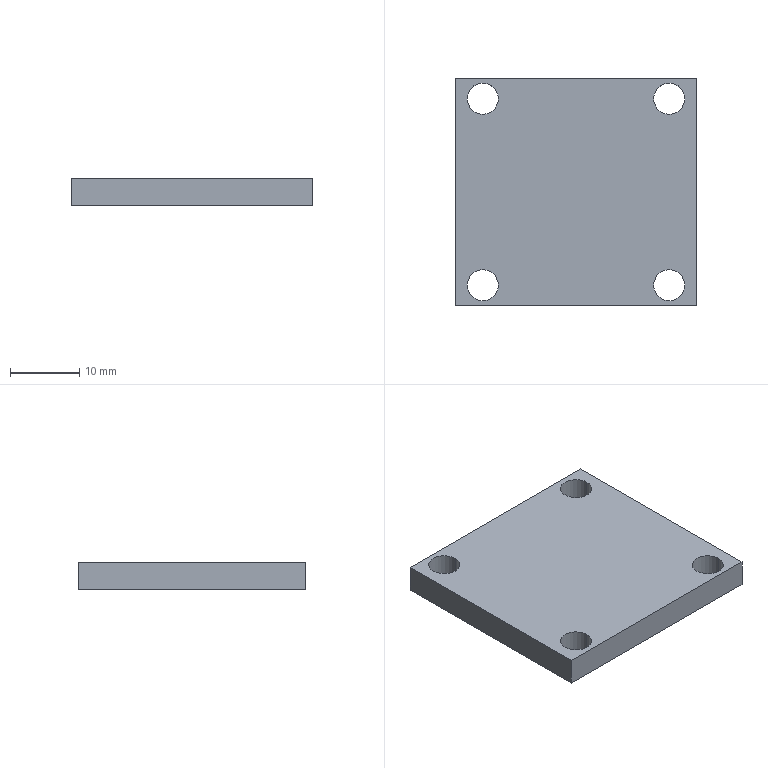Part | SolidWorks | features Extrusion 1, HoleWzd 1 | 1 solid | 14 faces | box 35 x 33 x 4 mm | volume 4366 mm3 | cylinder 8 | plane 6 | commonest cylinder face diameters 4.5 x8
STEP:
#1=CARTESIAN_POINT('',(11.25,13.5,0.));
#2=VERTEX_POINT('',#1);
#3=CARTESIAN_POINT('',(15.75,13.5,0.));
#4=VERTEX_POINT('',#3);
#5=CARTESIAN_POINT('',(13.5,13.5,0.));
#6=DIRECTION('',(0.,0.,1.));
#7=DIRECTION('',(1.,0.,0.));
#8=AXIS2_PLACEMENT_3D('',#5,#6,#7);
#9=CIRCLE('',#8,2.25);
#10=EDGE_CURVE('',#2,#4,#9,.T.);
#11=ORIENTED_EDGE('',*,*,#10,.F.);
#12=CARTESIAN_POINT('',(11.25,13.5,4.));
#13=VERTEX_POINT('',#12);
#14=CARTESIAN_POINT('',(11.25,13.5,4.));
#15=DIRECTION('',(0.,0.,1.));
#16=VECTOR('',#15,1000.);
#17=LINE('',#14,#16);
#18=EDGE_CURVE('',#2,#13,#17,.T.);
#19=ORIENTED_EDGE('',*,*,#18,.T.);
#20=CARTESIAN_POINT('',(15.75,13.5,4.));
#21=VERTEX_POINT('',#20);
#22=CARTESIAN_POINT('',(13.5,13.5,4.));
#23=DIRECTION('',(0.,0.,1.));
#24=DIRECTION('',(1.,0.,0.));
#25=AXIS2_PLACEMENT_3D('',#22,#23,#24);
#26=CIRCLE('',#25,2.25);
#27=EDGE_CURVE('',#13,#21,#26,.T.);
#28=ORIENTED_EDGE('',*,*,#27,.T.);
#29=CARTESIAN_POINT('',(15.75,13.5,4.));
#30=DIRECTION('',(0.,0.,1.));
#31=VECTOR('',#30,1000.);
#32=LINE('',#29,#31);
#33=EDGE_CURVE('',#4,#21,#32,.T.);
#34=ORIENTED_EDGE('',*,*,#33,.F.);
#35=EDGE_LOOP('',(#11,#19,#28,#34));
#36=FACE_OUTER_BOUND('',#35,.T.);
#37=CARTESIAN_POINT('',(13.5,13.5,4.));
#38=DIRECTION('',(0.,0.,1.));
#39=DIRECTION('',(1.,0.,0.));
#40=AXIS2_PLACEMENT_3D('',#37,#38,#39);
#41=CYLINDRICAL_SURFACE('',#40,2.25);
#42=ADVANCED_FACE('',(#36),#41,.F.);
#43=CARTESIAN_POINT('',(-15.75,13.5,0.));
#44=VERTEX_POINT('',#43);
#45=CARTESIAN_POINT('',(-11.25,13.5,0.));
#46=VERTEX_POINT('',#45);
#47=CARTESIAN_POINT('',(-13.5,13.5,0.));
#48=DIRECTION('',(0.,0.,1.));
#49=DIRECTION('',(1.,0.,0.));
#50=AXIS2_PLACEMENT_3D('',#47,#48,#49);
#51=CIRCLE('',#50,2.25);
#52=EDGE_CURVE('',#44,#46,#51,.T.);
#53=ORIENTED_EDGE('',*,*,#52,.F.);
#54=CARTESIAN_POINT('',(-15.75,13.5,4.));
#55=VERTEX_POINT('',#54);
#56=CARTESIAN_POINT('',(-15.75,13.5,4.));
#57=DIRECTION('',(0.,0.,1.));
#58=VECTOR('',#57,1000.);
#59=LINE('',#56,#58);
#60=EDGE_CURVE('',#44,#55,#59,.T.);
#61=ORIENTED_EDGE('',*,*,#60,.T.);
#62=CARTESIAN_POINT('',(-11.25,13.5,4.));
#63=VERTEX_POINT('',#62);
#64=CARTESIAN_POINT('',(-13.5,13.5,4.));
#65=DIRECTION('',(0.,0.,1.));
#66=DIRECTION('',(1.,0.,0.));
#67=AXIS2_PLACEMENT_3D('',#64,#65,#66);
#68=CIRCLE('',#67,2.25);
#69=EDGE_CURVE('',#55,#63,#68,.T.);
#70=ORIENTED_EDGE('',*,*,#69,.T.);
#71=CARTESIAN_POINT('',(-11.25,13.5,4.));
#72=DIRECTION('',(0.,0.,1.));
#73=VECTOR('',#72,1000.);
#74=LINE('',#71,#73);
#75=EDGE_CURVE('',#46,#63,#74,.T.);
#76=ORIENTED_EDGE('',*,*,#75,.F.);
#77=EDGE_LOOP('',(#53,#61,#70,#76));
#78=FACE_OUTER_BOUND('',#77,.T.);
#79=CARTESIAN_POINT('',(-13.5,13.5,4.));
#80=DIRECTION('',(0.,0.,1.));
#81=DIRECTION('',(1.,0.,0.));
#82=AXIS2_PLACEMENT_3D('',#79,#80,#81);
#83=CYLINDRICAL_SURFACE('',#82,2.25);
#84=ADVANCED_FACE('',(#78),#83,.F.);
#85=CARTESIAN_POINT('',(-15.75,-13.5,0.));
#86=VERTEX_POINT('',#85);
#87=CARTESIAN_POINT('',(-11.25,-13.5,0.));
#88=VERTEX_POINT('',#87);
#89=CARTESIAN_POINT('',(-13.5,-13.5,0.));
#90=DIRECTION('',(0.,0.,1.));
#91=DIRECTION('',(1.,0.,0.));
#92=AXIS2_PLACEMENT_3D('',#89,#90,#91);
#93=CIRCLE('',#92,2.25);
#94=EDGE_CURVE('',#86,#88,#93,.T.);
#95=ORIENTED_EDGE('',*,*,#94,.F.);
#96=CARTESIAN_POINT('',(-15.75,-13.5,4.));
#97=VERTEX_POINT('',#96);
#98=CARTESIAN_POINT('',(-15.75,-13.5,4.));
#99=DIRECTION('',(0.,0.,1.));
#100=VECTOR('',#99,1000.);
#101=LINE('',#98,#100);
#102=EDGE_CURVE('',#86,#97,#101,.T.);
#103=ORIENTED_EDGE('',*,*,#102,.T.);
#104=CARTESIAN_POINT('',(-11.25,-13.5,4.));
#105=VERTEX_POINT('',#104);
#106=CARTESIAN_POINT('',(-13.5,-13.5,4.));
#107=DIRECTION('',(0.,0.,1.));
#108=DIRECTION('',(1.,0.,0.));
#109=AXIS2_PLACEMENT_3D('',#106,#107,#108);
#110=CIRCLE('',#109,2.25);
#111=EDGE_CURVE('',#97,#105,#110,.T.);
#112=ORIENTED_EDGE('',*,*,#111,.T.);
#113=CARTESIAN_POINT('',(-11.25,-13.5,4.));
#114=DIRECTION('',(0.,0.,1.));
#115=VECTOR('',#114,1000.);
#116=LINE('',#113,#115);
#117=EDGE_CURVE('',#88,#105,#116,.T.);
#118=ORIENTED_EDGE('',*,*,#117,.F.);
#119=EDGE_LOOP('',(#95,#103,#112,#118));
#120=FACE_OUTER_BOUND('',#119,.T.);
#121=CARTESIAN_POINT('',(-13.5,-13.5,4.));
#122=DIRECTION('',(0.,0.,1.));
#123=DIRECTION('',(1.,0.,0.));
#124=AXIS2_PLACEMENT_3D('',#121,#122,#123);
#125=CYLINDRICAL_SURFACE('',#124,2.25);
#126=ADVANCED_FACE('',(#120),#125,.F.);
#127=CARTESIAN_POINT('',(11.25,-13.5,0.));
#128=VERTEX_POINT('',#127);
#129=CARTESIAN_POINT('',(15.75,-13.5,0.));
#130=VERTEX_POINT('',#129);
#131=CARTESIAN_POINT('',(13.5,-13.5,0.));
#132=DIRECTION('',(0.,0.,1.));
#133=DIRECTION('',(1.,0.,0.));
#134=AXIS2_PLACEMENT_3D('',#131,#132,#133);
#135=CIRCLE('',#134,2.25);
#136=EDGE_CURVE('',#128,#130,#135,.T.);
#137=ORIENTED_EDGE('',*,*,#136,.F.);
#138=CARTESIAN_POINT('',(11.25,-13.5,4.));
#139=VERTEX_POINT('',#138);
#140=CARTESIAN_POINT('',(11.25,-13.5,4.));
#141=DIRECTION('',(0.,0.,1.));
#142=VECTOR('',#141,1000.);
#143=LINE('',#140,#142);
#144=EDGE_CURVE('',#128,#139,#143,.T.);
#145=ORIENTED_EDGE('',*,*,#144,.T.);
#146=CARTESIAN_POINT('',(15.75,-13.5,4.));
#147=VERTEX_POINT('',#146);
#148=CARTESIAN_POINT('',(13.5,-13.5,4.));
#149=DIRECTION('',(0.,0.,1.));
#150=DIRECTION('',(1.,0.,0.));
#151=AXIS2_PLACEMENT_3D('',#148,#149,#150);
#152=CIRCLE('',#151,2.25);
#153=EDGE_CURVE('',#139,#147,#152,.T.);
#154=ORIENTED_EDGE('',*,*,#153,.T.);
#155=CARTESIAN_POINT('',(15.75,-13.5,4.));
#156=DIRECTION('',(0.,0.,1.));
#157=VECTOR('',#156,1000.);
#158=LINE('',#155,#157);
#159=EDGE_CURVE('',#130,#147,#158,.T.);
#160=ORIENTED_EDGE('',*,*,#159,.F.);
#161=EDGE_LOOP('',(#137,#145,#154,#160));
#162=FACE_OUTER_BOUND('',#161,.T.);
#163=CARTESIAN_POINT('',(13.5,-13.5,4.));
#164=DIRECTION('',(0.,0.,1.));
#165=DIRECTION('',(1.,0.,0.));
#166=AXIS2_PLACEMENT_3D('',#163,#164,#165);
#167=CYLINDRICAL_SURFACE('',#166,2.25);
#168=ADVANCED_FACE('',(#162),#167,.F.);
#169=CARTESIAN_POINT('',(17.5,-16.5,0.));
#170=VERTEX_POINT('',#169);
#171=CARTESIAN_POINT('',(17.5,16.5,0.));
#172=VERTEX_POINT('',#171);
#173=CARTESIAN_POINT('',(17.5,16.5,0.));
#174=DIRECTION('',(0.,1.,0.));
#175=VECTOR('',#174,1000.);
#176=LINE('',#173,#175);
#177=EDGE_CURVE('',#170,#172,#176,.T.);
#178=ORIENTED_EDGE('',*,*,#177,.T.);
#179=CARTESIAN_POINT('',(17.5,16.5,4.));
#180=VERTEX_POINT('',#179);
#181=CARTESIAN_POINT('',(17.5,16.5,4.));
#182=DIRECTION('',(0.,0.,-1.));
#183=VECTOR('',#182,1000.);
#184=LINE('',#181,#183);
#185=EDGE_CURVE('',#180,#172,#184,.T.);
#186=ORIENTED_EDGE('',*,*,#185,.F.);
#187=CARTESIAN_POINT('',(17.5,-16.5,4.));
#188=VERTEX_POINT('',#187);
#189=CARTESIAN_POINT('',(17.5,16.5,4.));
#190=DIRECTION('',(0.,1.,0.));
#191=VECTOR('',#190,1000.);
#192=LINE('',#189,#191);
#193=EDGE_CURVE('',#188,#180,#192,.T.);
#194=ORIENTED_EDGE('',*,*,#193,.F.);
#195=CARTESIAN_POINT('',(17.5,-16.5,4.));
#196=DIRECTION('',(0.,0.,-1.));
#197=VECTOR('',#196,1000.);
#198=LINE('',#195,#197);
#199=EDGE_CURVE('',#188,#170,#198,.T.);
#200=ORIENTED_EDGE('',*,*,#199,.T.);
#201=EDGE_LOOP('',(#178,#186,#194,#200));
#202=FACE_OUTER_BOUND('',#201,.T.);
#203=CARTESIAN_POINT('',(17.5,16.5,4.));
#204=DIRECTION('',(-1.,0.,0.));
#205=DIRECTION('',(0.,-1.,0.));
#206=AXIS2_PLACEMENT_3D('',#203,#204,#205);
#207=PLANE('',#206);
#208=ADVANCED_FACE('',(#202),#207,.F.);
#209=CARTESIAN_POINT('',(-17.5,16.5,0.));
#210=VERTEX_POINT('',#209);
#211=CARTESIAN_POINT('',(-17.5,16.5,0.));
#212=DIRECTION('',(-1.,0.,0.));
#213=VECTOR('',#212,1000.);
#214=LINE('',#211,#213);
#215=EDGE_CURVE('',#172,#210,#214,.T.);
#216=ORIENTED_EDGE('',*,*,#215,.T.);
#217=CARTESIAN_POINT('',(-17.5,16.5,4.));
#218=VERTEX_POINT('',#217);
#219=CARTESIAN_POINT('',(-17.5,16.5,4.));
#220=DIRECTION('',(0.,0.,-1.));
#221=VECTOR('',#220,1000.);
#222=LINE('',#219,#221);
#223=EDGE_CURVE('',#218,#210,#222,.T.);
#224=ORIENTED_EDGE('',*,*,#223,.F.);
#225=CARTESIAN_POINT('',(-17.5,16.5,4.));
#226=DIRECTION('',(-1.,0.,0.));
#227=VECTOR('',#226,1000.);
#228=LINE('',#225,#227);
#229=EDGE_CURVE('',#180,#218,#228,.T.);
#230=ORIENTED_EDGE('',*,*,#229,.F.);
#231=ORIENTED_EDGE('',*,*,#185,.T.);
#232=EDGE_LOOP('',(#216,#224,#230,#231));
#233=FACE_OUTER_BOUND('',#232,.T.);
#234=CARTESIAN_POINT('',(-17.5,16.5,4.));
#235=DIRECTION('',(0.,-1.,0.));
#236=DIRECTION('',(0.,0.,-1.));
#237=AXIS2_PLACEMENT_3D('',#234,#235,#236);
#238=PLANE('',#237);
#239=ADVANCED_FACE('',(#233),#238,.F.);
#240=CARTESIAN_POINT('',(-17.5,-16.5,0.));
#241=VERTEX_POINT('',#240);
#242=CARTESIAN_POINT('',(-17.5,16.5,0.));
#243=DIRECTION('',(0.,-1.,0.));
#244=VECTOR('',#243,1000.);
#245=LINE('',#242,#244);
#246=EDGE_CURVE('',#210,#241,#245,.T.);
#247=ORIENTED_EDGE('',*,*,#246,.T.);
#248=CARTESIAN_POINT('',(-17.5,-16.5,4.));
#249=VERTEX_POINT('',#248);
#250=CARTESIAN_POINT('',(-17.5,-16.5,4.));
#251=DIRECTION('',(0.,0.,-1.));
#252=VECTOR('',#251,1000.);
#253=LINE('',#250,#252);
#254=EDGE_CURVE('',#249,#241,#253,.T.);
#255=ORIENTED_EDGE('',*,*,#254,.F.);
#256=CARTESIAN_POINT('',(-17.5,16.5,4.));
#257=DIRECTION('',(0.,-1.,0.));
#258=VECTOR('',#257,1000.);
#259=LINE('',#256,#258);
#260=EDGE_CURVE('',#218,#249,#259,.T.);
#261=ORIENTED_EDGE('',*,*,#260,.F.);
#262=ORIENTED_EDGE('',*,*,#223,.T.);
#263=EDGE_LOOP('',(#247,#255,#261,#262));
#264=FACE_OUTER_BOUND('',#263,.T.);
#265=CARTESIAN_POINT('',(-17.5,16.5,4.));
#266=DIRECTION('',(1.,0.,0.));
#267=DIRECTION('',(0.,1.,0.));
#268=AXIS2_PLACEMENT_3D('',#265,#266,#267);
#269=PLANE('',#268);
#270=ADVANCED_FACE('',(#264),#269,.F.);
#271=CARTESIAN_POINT('',(-17.5,-16.5,0.));
#272=DIRECTION('',(1.,0.,0.));
#273=VECTOR('',#272,1000.);
#274=LINE('',#271,#273);
#275=EDGE_CURVE('',#241,#170,#274,.T.);
#276=ORIENTED_EDGE('',*,*,#275,.T.);
#277=ORIENTED_EDGE('',*,*,#199,.F.);
#278=CARTESIAN_POINT('',(-17.5,-16.5,4.));
#279=DIRECTION('',(1.,0.,0.));
#280=VECTOR('',#279,1000.);
#281=LINE('',#278,#280);
#282=EDGE_CURVE('',#249,#188,#281,.T.);
#283=ORIENTED_EDGE('',*,*,#282,.F.);
#284=ORIENTED_EDGE('',*,*,#254,.T.);
#285=EDGE_LOOP('',(#276,#277,#283,#284));
#286=FACE_OUTER_BOUND('',#285,.T.);
#287=CARTESIAN_POINT('',(-17.5,-16.5,4.));
#288=DIRECTION('',(0.,1.,0.));
#289=DIRECTION('',(0.,0.,1.));
#290=AXIS2_PLACEMENT_3D('',#287,#288,#289);
#291=PLANE('',#290);
#292=ADVANCED_FACE('',(#286),#291,.F.);
#293=CARTESIAN_POINT('',(13.5,13.5,4.));
#294=DIRECTION('',(0.,0.,1.));
#295=DIRECTION('',(1.,0.,0.));
#296=AXIS2_PLACEMENT_3D('',#293,#294,#295);
#297=CIRCLE('',#296,2.25);
#298=EDGE_CURVE('',#21,#13,#297,.T.);
#299=ORIENTED_EDGE('',*,*,#298,.F.);
#300=ORIENTED_EDGE('',*,*,#27,.F.);
#301=EDGE_LOOP('',(#299,#300));
#302=FACE_BOUND('',#301,.T.);
#303=CARTESIAN_POINT('',(-13.5,13.5,4.));
#304=DIRECTION('',(0.,0.,1.));
#305=DIRECTION('',(1.,0.,0.));
#306=AXIS2_PLACEMENT_3D('',#303,#304,#305);
#307=CIRCLE('',#306,2.25);
#308=EDGE_CURVE('',#63,#55,#307,.T.);
#309=ORIENTED_EDGE('',*,*,#308,.F.);
#310=ORIENTED_EDGE('',*,*,#69,.F.);
#311=EDGE_LOOP('',(#309,#310));
#312=FACE_BOUND('',#311,.T.);
#313=CARTESIAN_POINT('',(-13.5,-13.5,4.));
#314=DIRECTION('',(0.,0.,1.));
#315=DIRECTION('',(1.,0.,0.));
#316=AXIS2_PLACEMENT_3D('',#313,#314,#315);
#317=CIRCLE('',#316,2.25);
#318=EDGE_CURVE('',#105,#97,#317,.T.);
#319=ORIENTED_EDGE('',*,*,#318,.F.);
#320=ORIENTED_EDGE('',*,*,#111,.F.);
#321=EDGE_LOOP('',(#319,#320));
#322=FACE_BOUND('',#321,.T.);
#323=CARTESIAN_POINT('',(13.5,-13.5,4.));
#324=DIRECTION('',(0.,0.,1.));
#325=DIRECTION('',(1.,0.,0.));
#326=AXIS2_PLACEMENT_3D('',#323,#324,#325);
#327=CIRCLE('',#326,2.25);
#328=EDGE_CURVE('',#147,#139,#327,.T.);
#329=ORIENTED_EDGE('',*,*,#328,.F.);
#330=ORIENTED_EDGE('',*,*,#153,.F.);
#331=EDGE_LOOP('',(#329,#330));
#332=FACE_BOUND('',#331,.T.);
#333=ORIENTED_EDGE('',*,*,#193,.T.);
#334=ORIENTED_EDGE('',*,*,#229,.T.);
#335=ORIENTED_EDGE('',*,*,#260,.T.);
#336=ORIENTED_EDGE('',*,*,#282,.T.);
#337=EDGE_LOOP('',(#333,#334,#335,#336));
#338=FACE_OUTER_BOUND('',#337,.T.);
#339=CARTESIAN_POINT('',(0.,0.,4.));
#340=DIRECTION('',(0.,0.,1.));
#341=DIRECTION('',(1.,0.,0.));
#342=AXIS2_PLACEMENT_3D('',#339,#340,#341);
#343=PLANE('',#342);
#344=ADVANCED_FACE('',(#302,#312,#322,#332,#338),#343,.T.);
#345=CARTESIAN_POINT('',(13.5,13.5,0.));
#346=DIRECTION('',(0.,0.,1.));
#347=DIRECTION('',(1.,0.,0.));
#348=AXIS2_PLACEMENT_3D('',#345,#346,#347);
#349=CIRCLE('',#348,2.25);
#350=EDGE_CURVE('',#4,#2,#349,.T.);
#351=ORIENTED_EDGE('',*,*,#350,.T.);
#352=ORIENTED_EDGE('',*,*,#10,.T.);
#353=EDGE_LOOP('',(#351,#352));
#354=FACE_BOUND('',#353,.T.);
#355=CARTESIAN_POINT('',(-13.5,13.5,0.));
#356=DIRECTION('',(0.,0.,1.));
#357=DIRECTION('',(1.,0.,0.));
#358=AXIS2_PLACEMENT_3D('',#355,#356,#357);
#359=CIRCLE('',#358,2.25);
#360=EDGE_CURVE('',#46,#44,#359,.T.);
#361=ORIENTED_EDGE('',*,*,#360,.T.);
#362=ORIENTED_EDGE('',*,*,#52,.T.);
#363=EDGE_LOOP('',(#361,#362));
#364=FACE_BOUND('',#363,.T.);
#365=CARTESIAN_POINT('',(-13.5,-13.5,0.));
#366=DIRECTION('',(0.,0.,1.));
#367=DIRECTION('',(1.,0.,0.));
#368=AXIS2_PLACEMENT_3D('',#365,#366,#367);
#369=CIRCLE('',#368,2.25);
#370=EDGE_CURVE('',#88,#86,#369,.T.);
#371=ORIENTED_EDGE('',*,*,#370,.T.);
#372=ORIENTED_EDGE('',*,*,#94,.T.);
#373=EDGE_LOOP('',(#371,#372));
#374=FACE_BOUND('',#373,.T.);
#375=CARTESIAN_POINT('',(13.5,-13.5,0.));
#376=DIRECTION('',(0.,0.,1.));
#377=DIRECTION('',(1.,0.,0.));
#378=AXIS2_PLACEMENT_3D('',#375,#376,#377);
#379=CIRCLE('',#378,2.25);
#380=EDGE_CURVE('',#130,#128,#379,.T.);
#381=ORIENTED_EDGE('',*,*,#380,.T.);
#382=ORIENTED_EDGE('',*,*,#136,.T.);
#383=EDGE_LOOP('',(#381,#382));
#384=FACE_BOUND('',#383,.T.);
#385=ORIENTED_EDGE('',*,*,#177,.F.);
#386=ORIENTED_EDGE('',*,*,#275,.F.);
#387=ORIENTED_EDGE('',*,*,#246,.F.);
#388=ORIENTED_EDGE('',*,*,#215,.F.);
#389=EDGE_LOOP('',(#385,#386,#387,#388));
#390=FACE_OUTER_BOUND('',#389,.T.);
#391=CARTESIAN_POINT('',(0.,0.,0.));
#392=DIRECTION('',(0.,0.,1.));
#393=DIRECTION('',(1.,0.,0.));
#394=AXIS2_PLACEMENT_3D('',#391,#392,#393);
#395=PLANE('',#394);
#396=ADVANCED_FACE('',(#354,#364,#374,#384,#390),#395,.F.);
#397=ORIENTED_EDGE('',*,*,#144,.F.);
#398=ORIENTED_EDGE('',*,*,#380,.F.);
#399=ORIENTED_EDGE('',*,*,#159,.T.);
#400=ORIENTED_EDGE('',*,*,#328,.T.);
#401=EDGE_LOOP('',(#397,#398,#399,#400));
#402=FACE_OUTER_BOUND('',#401,.T.);
#403=CARTESIAN_POINT('',(13.5,-13.5,4.));
#404=DIRECTION('',(0.,0.,1.));
#405=DIRECTION('',(1.,0.,0.));
#406=AXIS2_PLACEMENT_3D('',#403,#404,#405);
#407=CYLINDRICAL_SURFACE('',#406,2.25);
#408=ADVANCED_FACE('',(#402),#407,.F.);
#409=ORIENTED_EDGE('',*,*,#102,.F.);
#410=ORIENTED_EDGE('',*,*,#370,.F.);
#411=ORIENTED_EDGE('',*,*,#117,.T.);
#412=ORIENTED_EDGE('',*,*,#318,.T.);
#413=EDGE_LOOP('',(#409,#410,#411,#412));
#414=FACE_OUTER_BOUND('',#413,.T.);
#415=CARTESIAN_POINT('',(-13.5,-13.5,4.));
#416=DIRECTION('',(0.,0.,1.));
#417=DIRECTION('',(1.,0.,0.));
#418=AXIS2_PLACEMENT_3D('',#415,#416,#417);
#419=CYLINDRICAL_SURFACE('',#418,2.25);
#420=ADVANCED_FACE('',(#414),#419,.F.);
#421=ORIENTED_EDGE('',*,*,#60,.F.);
#422=ORIENTED_EDGE('',*,*,#360,.F.);
#423=ORIENTED_EDGE('',*,*,#75,.T.);
#424=ORIENTED_EDGE('',*,*,#308,.T.);
#425=EDGE_LOOP('',(#421,#422,#423,#424));
#426=FACE_OUTER_BOUND('',#425,.T.);
#427=CARTESIAN_POINT('',(-13.5,13.5,4.));
#428=DIRECTION('',(0.,0.,1.));
#429=DIRECTION('',(1.,0.,0.));
#430=AXIS2_PLACEMENT_3D('',#427,#428,#429);
#431=CYLINDRICAL_SURFACE('',#430,2.25);
#432=ADVANCED_FACE('',(#426),#431,.F.);
#433=ORIENTED_EDGE('',*,*,#18,.F.);
#434=ORIENTED_EDGE('',*,*,#350,.F.);
#435=ORIENTED_EDGE('',*,*,#33,.T.);
#436=ORIENTED_EDGE('',*,*,#298,.T.);
#437=EDGE_LOOP('',(#433,#434,#435,#436));
#438=FACE_OUTER_BOUND('',#437,.T.);
#439=CARTESIAN_POINT('',(13.5,13.5,4.));
#440=DIRECTION('',(0.,0.,1.));
#441=DIRECTION('',(1.,0.,0.));
#442=AXIS2_PLACEMENT_3D('',#439,#440,#441);
#443=CYLINDRICAL_SURFACE('',#442,2.25);
#444=ADVANCED_FACE('',(#438),#443,.F.);
#445=CLOSED_SHELL('',(#42,#84,#126,#168,#208,#239,#270,#292,#344,#396,#408,#420,#432,#444));
#446=MANIFOLD_SOLID_BREP('',#445);
#447=CARTESIAN_POINT('',(0.,0.,0.));
#448=DIRECTION('',(0.,0.,1.));
#449=DIRECTION('',(1.,0.,0.));
#450=AXIS2_PLACEMENT_3D('',#447,#448,#449);
#451=(LENGTH_UNIT()NAMED_UNIT(*)SI_UNIT(.MILLI.,.METRE.));
#452=UNCERTAINTY_MEASURE_WITH_UNIT(LENGTH_MEASURE(0.00001),#451,'','');
#453=(NAMED_UNIT(*)PLANE_ANGLE_UNIT()SI_UNIT($,.RADIAN.));
#454=(NAMED_UNIT(*)SI_UNIT($,.STERADIAN.)SOLID_ANGLE_UNIT());
#455=(GEOMETRIC_REPRESENTATION_CONTEXT(3)GLOBAL_UNCERTAINTY_ASSIGNED_CONTEXT((#452))GLOBAL_UNIT_ASSIGNED_CONTEXT((#451,#453,#454))REPRESENTATION_CONTEXT('',''));
#456=ADVANCED_BREP_SHAPE_REPRESENTATION('',(#446,#450),#455);